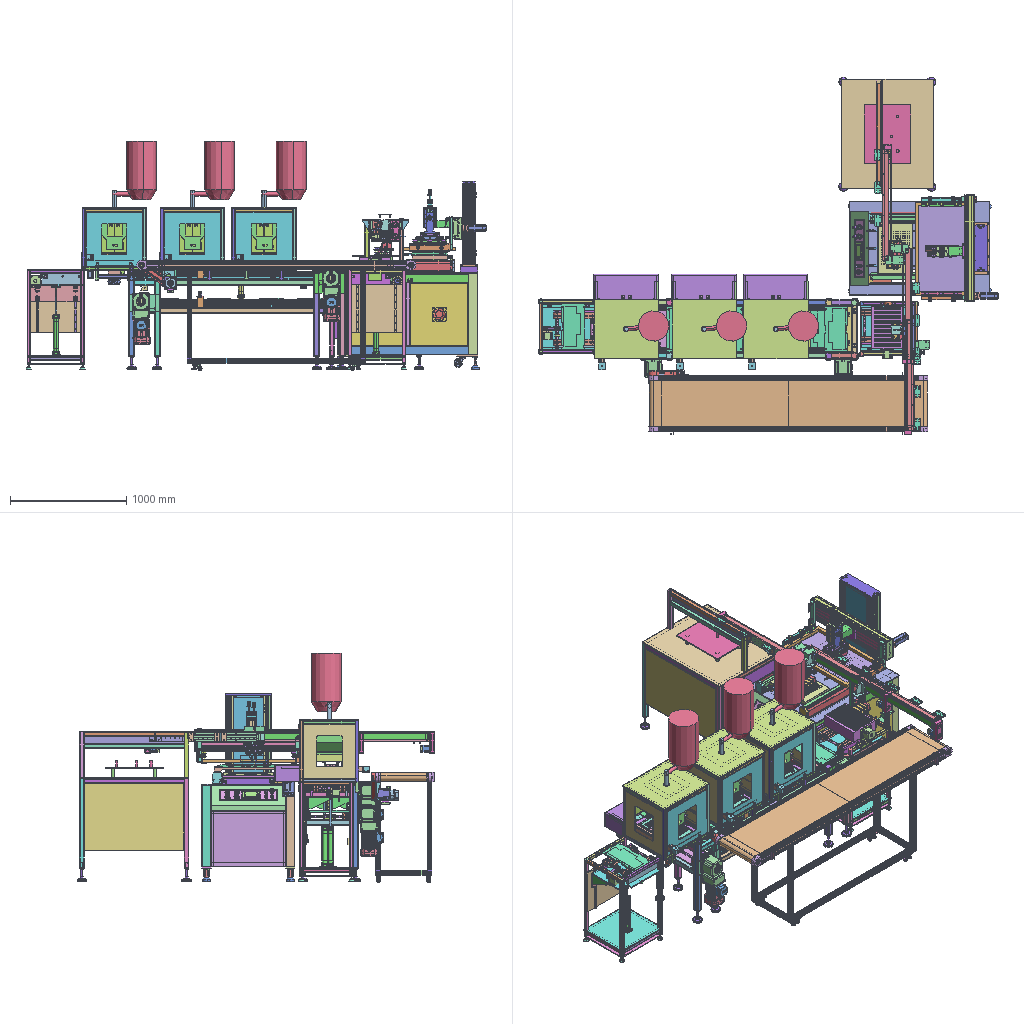Assembly | STEP file | 266 different items | 841 placed | box 3950 x 3072 x 1968 mm
Parts list (item | name | quantity | parent item | size | volume):
1 | 001. Pressure gauge (without flange) | x2 | in Circuit control assembly | 42 x 42 x 38 mm | 32331 mm3
2 | 001. Schneider red emergency stop switch XB2-BS542C | x1 | in Circuit control assembly | 40 x 40 x 49 mm | 26880 mm3
3 | 001. Schneider two-position switch XB2-BD21C | x2 | in Circuit control assembly | 28.3 x 29.2 x 44.3 mm | 13844 mm3
4 | 001. Yiweide green push-button switch EB6-BA31 | x1 | in Circuit control assembly | 28.3 x 28.3 x 27.1 mm | 9249 mm3
5 | 1.6 m_VMF01-40-4-A-001 | x27 | in 1.6米VMF01-40-2-A | 18.36 x 10.41 x 23.11 mm | 962.85 mm3
6 | 1.6 m_VMF01-40-4-A-002 | x27 | in 1.6米VMF01-40-2-A | 11.17 x 12.07 x 24.77 mm | 1310 mm3
7 | 1.6米90W | x1 | in MYT-A01-13 | 160.5 x 104 x 90 mm | 953973 mm3
8 | 1.6米B6204ZZ | x4 | in MYT-A01-13 | 14 x 47 x 47 mm | 19015 mm3
9 | 1.6米HFS8-4040-110 | x4 | in MYT-A01-13 | 40 x 40 x 800 mm | 497640 mm3
10 | 1.6米HFS8-4040-2150 | x2 | in MYT-A01-13 | 40 x 40 x 1450 mm | 901973 mm3
11 | 1.6米HFS8-4040-400 | x2 | in MYT-A01-13 | 40 x 40 x 400 mm | 248820 mm3
12 | 1.6米HFS8-4080-3000 | x2 | in MYT-A01-13 | 40 x 80 x 2230 mm | 2325189 mm3
13 | 1.6米L型片 | x4 | in MYT-A01-13 | 27 x 80 x 27 mm | 11342 mm3
14 | 1.6米VLF02-40-10-D15 | x2 | in MYT-A01-13 | 46 x 44.551 x 22 mm | 14102 mm3
15 | 1.6米托片 | x2 | in MYT-A01-13 | 49 x 32 x 36 mm | 5023 mm3
16 | 1.6米滚轮1 | x1 | in MYT-A01-13 | 70 x 486 x 70 mm | 1669260 mm3
17 | 1.6米滚轮2 | x1 | in MYT-A01-13 | 70 x 516 x 70 mm | 1674212 mm3
18 | 1.6米Belt | x1 | in MYT-A01-13 | 2391 x 398 x 76 mm | 5802047 mm3
19 | 1.6米Belt线支撑(Default) | x2 | in MYT-A01-13 | 400 x 1085 x 40 mm | 772332 mm3
20 | 1.6米Belt罩 | x1 | in MYT-A01-13 | 359.4 x 80 x 39 mm | 70115 mm3
21 | 1.6米脚轮垫块 | x4 | in MYT-A01-13 | 99 x 5 x 50 mm | 23511 mm3
22 | 1.6米轴承套 | x4 | in MYT-A01-13 | 53 x 25 x 53 mm | 15579 mm3
23 | 1.6米轴盖 | x4 | in MYT-A01-13 | 195 x 67 x 85 mm | 66626 mm3
24 | 1.6米马达罩 | x1 | in MYT-A01-13 | 145 x 105 x 42 mm | 63685 mm3
25 | 10 | x8 | in MHC-H24-2-L410 Shanglong slider, MHC-H24-2-L410 Upper隆滑块-1, MHC-H24-2-L410 Upper隆滑块-2, MHC-H24-2-L410 Upper隆滑块-3, MHC-H24-2-L410 Upper隆滑块-4, MHC-H24-2-L410 Upper隆滑块-5, MHC-H24-2-L410 Upper隆滑块-6, MHC-H24-2-L410 Upper隆滑块-7 | 32 x 18.8 x 1 mm | 485.961 mm3
26 | 11 | x8 | in MHC-H24-2-L410 Shanglong slider, MHC-H24-2-L410 Upper隆滑块-1, MHC-H24-2-L410 Upper隆滑块-2, MHC-H24-2-L410 Upper隆滑块-3, MHC-H24-2-L410 Upper隆滑块-4, MHC-H24-2-L410 Upper隆滑块-5, MHC-H24-2-L410 Upper隆滑块-6, MHC-H24-2-L410 Upper隆滑块-7 | 32 x 19.4 x 7.5 mm | 2771 mm3
27 | 12 | x8 | in MHC-H24-2-L410 Shanglong slider, MHC-H24-2-L410 Upper隆滑块-1, MHC-H24-2-L410 Upper隆滑块-2, MHC-H24-2-L410 Upper隆滑块-3, MHC-H24-2-L410 Upper隆滑块-4, MHC-H24-2-L410 Upper隆滑块-5, MHC-H24-2-L410 Upper隆滑块-6, MHC-H24-2-L410 Upper隆滑块-7 | 32 x 18.8 x 1 mm | 479.678 mm3
28 | 13 | x8 | in MHC-H24-2-L410 Shanglong slider, MHC-H24-2-L410 Upper隆滑块-1, MHC-H24-2-L410 Upper隆滑块-2, MHC-H24-2-L410 Upper隆滑块-3, MHC-H24-2-L410 Upper隆滑块-4, MHC-H24-2-L410 Upper隆滑块-5, MHC-H24-2-L410 Upper隆滑块-6, MHC-H24-2-L410 Upper隆滑块-7 | 7.302 x 8 x 6.95 mm | 149.976 mm3
29 | 200ys04 | x3 | in MYT-A01-06, MYT-A01-06-1, MYT-A01-06-2 | 199 x 143.386 x 105.972 mm | 487784 mm3
30 | 6022ZZ deep groove ball bearing MISUMI 62 | x4 | in Flat belt conveyor assembly, 平Belt输送Component-1 | 44 x 44 x 12 mm | 13685 mm3
31 | 8 | x8 | in MHC-H24-2-L410 Shanglong slider, MHC-H24-2-L410 Upper隆滑块-1, MHC-H24-2-L410 Upper隆滑块-2, MHC-H24-2-L410 Upper隆滑块-3, MHC-H24-2-L410 Upper隆滑块-4, MHC-H24-2-L410 Upper隆滑块-5, MHC-H24-2-L410 Upper隆滑块-6, MHC-H24-2-L410 Upper隆滑块-7 | 34 x 19.5 x 39.8 mm | 15652 mm3
32 | 866-BDO024-91-11A_default_machined_ | x9 | in 866-BDO024-95-00A_material release position, 866-BDO024-95-00A_放料位-1, 866-BDO024-95-00A_放料位-2 | 90 x 65 x 100 mm | 167392 mm3
33 | 866-BDO024-93-03A | x3 | in 866-BDO024-95-00A_material release position, 866-BDO024-95-00A_放料位-1, 866-BDO024-95-00A_放料位-2 | 80 x 61.5 x 14 mm | 48551 mm3
34 | 866-BDO024-93-04A | x3 | in 866-BDO024-95-00A_material release position, 866-BDO024-95-00A_放料位-1, 866-BDO024-95-00A_放料位-2 | 80 x 57 x 75 mm | 148857 mm3
35 | 866-BDO024-93-10A | x3 | in 866-BDO024-95-00A_material release position, 866-BDO024-95-00A_放料位-1, 866-BDO024-95-00A_放料位-2 | 16 x 35 x 9 mm | 897.701 mm3
36 | 866-BDO024-93-11A | x9 | in 866-BDO024-95-00A_material release position, 866-BDO024-95-00A_放料位-1, 866-BDO024-95-00A_放料位-2 | 25 x 6 x 3 mm | 420.548 mm3
37 | 866-BDO024-93-12A | x6 | in 866-BDO024-95-00A_material release position, 866-BDO024-95-00A_放料位-1, 866-BDO024-95-00A_放料位-2 | 80 x 61.5 x 20 mm | 50514 mm3
38 | 866-BDO024-95-01A_default | x3 | in 866-BDO024-95-00A_material release position, 866-BDO024-95-00A_放料位-1, 866-BDO024-95-00A_放料位-2 | 954 x 15 x 80 mm | 1055067 mm3
39 | 866-BDO024-95-03A | x3 | in 866-BDO024-95-00A_material release position, 866-BDO024-95-00A_放料位-1, 866-BDO024-95-00A_放料位-2 | 954 x 8 x 56 mm | 95867 mm3
40 | 866-BDO024-95-04A | x3 | in 866-BDO024-95-00A_material release position, 866-BDO024-95-00A_放料位-1, 866-BDO024-95-00A_放料位-2 | 942 x 56.5 x 13.5 mm | 95046 mm3
41 | 866-BDO024-95-05A | x3 | in 866-BDO024-95-00A_material release position, 866-BDO024-95-00A_放料位-1, 866-BDO024-95-00A_放料位-2 | 180 x 63 x 20 mm | 101274 mm3
42 | 866-BDO024-95-06A | x3 | in 866-BDO024-95-00A_material release position, 866-BDO024-95-00A_放料位-1, 866-BDO024-95-00A_放料位-2 | 66 x 46.5 x 183 mm | 47761 mm3
43 | 866-BDO024-95-07A_default | x3 | in 866-BDO024-95-00A_material release position, 866-BDO024-95-00A_放料位-1, 866-BDO024-95-00A_放料位-2 | 13.5 x 56.5 x 954 mm | 96451 mm3
44 | 866-BDO024-96-03A_default | x3 | in 866-BDO024-96-00A_material release position, 866-BDO024-96-00A_放料位-1, 866-BDO024-96-00A_放料位-2 | 148.5 x 75 x 45.5 mm | 21210 mm3
45 | 9 | x8 | in MHC-H24-2-L410 Shanglong slider, MHC-H24-2-L410 Upper隆滑块-1, MHC-H24-2-L410 Upper隆滑块-2, MHC-H24-2-L410 Upper隆滑块-3, MHC-H24-2-L410 Upper隆滑块-4, MHC-H24-2-L410 Upper隆滑块-5, MHC-H24-2-L410 Upper隆滑块-6, MHC-H24-2-L410 Upper隆滑块-7 | 32 x 19.4 x 7.5 mm | 2771 mm3
46 | 90yt01-18 | x1 | in Speed control motor assembly | - | -
47 | AC motor fixing | x1 | in Speed control motor assembly | 100 x 250 x 8 mm | 168414 mm3
48 | AJC-D48-M10-L80 | x8 | in AJC-D48-M10-L80 leveling foot cup Shanglong 17.2, AJC-D48-M10-L80 leveling foot cup Shanglong 17.2-1, AJC-D48-M10-L80 leveling foot cup Shanglong 17.2-2, AJC-D48-M10-L80 leveling foot cup Shanglong 17.2-3, AJC-D48-M10-L80 leveling foot cup Shanglong 17.2-4, AJC-D48-M10-L80 leveling foot cup Shanglong 17.2-5, AJC-D48-M10-L80 leveling foot cup Shanglong 17.2-6, AJC-D48-M10-L80 leveling foot cup Shanglong 17.2-7 | 48 x 102 x 48 mm | 30151 mm3
49 | AKQ41-G-Z-6065 | x12 | in MYT-A01-06, MYT-A01-06-1, MYT-A01-06-2 | 60 x 13.5 x 65 mm | 16186 mm3
50 | Air cylinder ACQJ-25X35-20_4_1-5 | x2 | in New head | 40 x 151.001 x 42 mm | 88087 mm3
51 | BAF629ZZ-E | x6 | in MYT-A01-06, MYT-A01-06-1, MYT-A01-06-2 | 8 x 26 x 26 mm | 3194 mm3
52 | BRTA-20 pillow block bearing Shanglong | x6 | in MYT-A01-00, MYT-A01-03, MYT-A01-03-1 | 37 x 73.015 x 127 mm | 112012 mm3
53 | BTL-01-32-0 | x4 | in MYT-A01-01, MYT-A01-01-1, MYT-A01-01-2, MYT-A01-01-3 | 40 x 32 x 32 mm | 13951 mm3
54 | Ball screw 4R16-16S2-DFSH-920-982-0.05(R)_HIWIN | x3 | in 866-BDO024-95-00A_material release position, 866-BDO024-95-00A_放料位-1, 866-BDO024-95-00A_放料位-2 | 982 x 16 x 16 mm | 189994 mm3
55 | Ball screw 4R16-16S2-DFSH-920-982-0.05(S)_HIWEI_default | x3 | in 866-BDO024-95-00A_material release position, 866-BDO024-95-00A_放料位-1, 866-BDO024-95-00A_放料位-2 | 38 x 53 x 48 mm | 38522 mm3
56 | Bearing B6000ZZ_MISUMI | x3 | in 866-BDO024-95-00A_material release position, 866-BDO024-95-00A_放料位-1, 866-BDO024-95-00A_放料位-2 | 8 x 26 x 26 mm | 2470 mm3
57 | Bearing B6201ZZNR_MISUMI | x6 | in 866-BDO024-95-00A_material release position, 866-BDO024-95-00A_放料位-1, 866-BDO024-95-00A_放料位-2 | 10 x 36.7 x 36.7 mm | 5407 mm3
58 | Blade clamp | x1 | in Blade-modified | 250 x 36 x 53 mm | 139062 mm3
59 | Blade fixing rod | x2 | in Blade-modified, 回墨刀-350 | 230 x 30 x 30 mm | 83181 mm3
60 | Blade holder 1 | x4 | in New head | 45 x 20 x 75 mm | 28350 mm3
61 | C-type retaining ring STWS10_MISUMI_default | x3 | in 866-BDO024-95-00A_material release position, 866-BDO024-95-00A_放料位-1, 866-BDO024-95-00A_放料位-2 | 12 x 1 x 14.09 mm | 51.059 mm3
62 | CA2F40-50Z_0_0_0_ | x1 | in MYT-A01-07 | 196 x 71 x 100 mm | 325906 mm3
63 | CA2G40-250Z_0_0_0_ | x2 | in MYT-A01-05, MYT-A01-05-1 | 624.042 x 71 x 100 mm | 473090 mm3
64 | CJ2KD16-45S_0_0_0_ | x3 | in MYT-A01-06, MYT-A01-06-1, MYT-A01-06-2 | 149 x 18.3 x 22.7 mm | 23348 mm3
65 | CQ2F16-20D_0_0_0_ | x6 | in MYT-A01-08, MYT-A01-08-1, MYT-A01-08-2, MYT-A01-08-3, MYT-A01-08-4 | 52 x 30 x 55 mm | 31057 mm3
66 | CQ2G32-50DZ_0_0_0_ | x3 | in MYT-A01-11, MYT-A01-11-1 | 88 x 51 x 65 mm | 108830 mm3
67 | Caster plate | x4 | in CMAZ40-N ultra-light caster, CMAZ40-N脚轮超轻载-1, CMAZ40-N脚轮超轻载-2, CMAZ40-N脚轮超轻载-3 | 50 x 6.8 x 69 mm | 8896 mm3
68 | Column | x2 | in Vertical arm unit | 107.4 x 51 x 700 mm | 1396461 mm3
69 | Column base plate | x1 | in Vertical arm unit | 450 x 150 x 15 mm | 884150 mm3
70 | Column cover plate | x1 | in Vertical arm unit | 400 x 107.5 x 15 mm | 621699 mm3
71 | Connecting bolt | x2 | in New head | 14 x 16.166 x 28 mm | 2024 mm3
72 | profile cover | x2 | in Blade-modified | 8 x 30 x 30 mm | 5851 mm3
73 | rotating shaft | x2 | in Blade clamp assembly, 刮刀夹组合-1 | 20 x 20 x 114 mm | 37100 mm3
74 | Crossbeam front guard plate | x1 | in Printing crossbeam unit | 98 x 8 x 898 mm | 149433 mm3
75 | Crossbeam slider connecting plate | x1 | in Printing crossbeam unit | 130 x 125 x 21 mm | 162372 mm3
76 | Double-speed chain return rail VMH01-BS25-C206B Yihda 124-0 | x6 | in MYT-A01-00, MYT-A01-03, MYT-A01-03-1 | 34 x 56.925 x 56.925 mm | 78739 mm3
77 | Driven wheel | x1 | in Driven wheel assembly | 42.62 x 42.62 x 24.392 mm | 14671 mm3
78 | Driven wheel shaft^Driven wheel assembly | x1 | in Driven wheel assembly | 16 x 16 x 66 mm | 7306 mm3
79 | Driving wheel | x1 | in Printing motor assembly | 42.62 x 42.62 x 24.392 mm | 18419 mm3
80 | E-LME12-d10 | x4 | in MYT-A01-07 | 29 x 40 x 40 mm | 8759 mm3
81 | E-WAC53-D80-M16-L125 | x12 | in MYT-A01-00, MYT-A01-09 | 80 x 165 x 80 mm | 107171 mm3
82 | EME01-W50-L0.793 flat belt Yihda 113 | x4 | in Flat belt conveyor assembly, 平Belt输送Component-1 | 362.8 x 62.8 x 50 mm | 76314 mm3
83 | ENE11-D60-N20-L50-X14-Y12-Z5 flat belt pulley Yihda 171 | x4 | in Flat belt conveyor assembly, 平Belt输送Component-1 | 60 x 60 x 50 mm | 110095 mm3
84 | ENJ11-D60-d20-L50-X14-Y12-Z5 flat belt idler Yihda 271 | x8 | in Flat belt idler assembly, 平带惰轮Component-1, 平带惰轮Component-2, 平带惰轮Component-3, 平带惰轮Component-4, 平带惰轮Component-5, 平带惰轮Component-6, 平带惰轮Component-7 | 60 x 60 x 50 mm | 111446 mm3
85 | Electromagnet | x2 | in Dual platform unit | 25 x 25 x 15 mm | 6939 mm3
86 | Five-star handle (with gland) (M10_40_40) | x3 | in Right screen clamp assembly^Screen assembly_PS-3045E-LDJ | 38.486 x 37.046 x 70.083 mm | 22563 mm3
87 | Five-star handle (with gland) 2 (M10_40_40) | x3 | in Right screen clamp assembly^Screen assembly_PS-3045E-LDJ2 | 38.486 x 37.046 x 70.083 mm | 22563 mm3
88 | Fixed seat | x1 | in New head | 105 x 75 x 160 mm | 453829 mm3
89 | Flat belt conveyor base plate | x2 | in Flat belt conveyor assembly, 平Belt输送Component-1 | 463 x 393.9 x 10 mm | 1773598 mm3
90 | Flat belt drive shaft | x6 | in Flat belt conveyor assembly, 平Belt输送Component-1 | 283.4 x 22 x 22 mm | 95567 mm3
91 | Flat belt motor mounting plate | x2 | in Flat belt conveyor assembly, 平Belt输送Component-1 | 86 x 101 x 12 mm | 83890 mm3
92 | Flat belt mounting plate | x2 | in Flat belt conveyor assembly, 平Belt输送Component-1 | 355 x 95 x 16 mm | 507779 mm3
93 | Floating joint | x4 | in Flat belt conveyor assembly, New head, 平Belt输送Component-1 | 20 x 38 x 33 mm | 13622 mm3
94 | Floating joint mounting plate | x2 | in Flat belt conveyor assembly, 平Belt输送Component-1 | 38 x 75 x 18 mm | 24096 mm3
95 | Flow limiter AS2201F-01-06_SMC_22-01-06 | x6 | in 866-BDO024-96-00A_material release position, 866-BDO024-96-00A_放料位-1, 866-BDO024-96-00A_放料位-2 | 27.5 x 36.1 x 14.2 mm | 4282 mm3
96 | Foot caster | x4 | in Frame unit | 60 x 96 x 114 mm | 163326 mm3
97 | Foot pad shim | x4 | in Foot cup, 地脚杯-1, 地脚杯-2, 地脚杯-3 | 65 x 65 x 35 mm | 88423 mm3
98 | Foot screw | x4 | in Foot cup, 地脚杯-1, 地脚杯-2, 地脚杯-3 | 20 x 118 x 20 mm | 31335 mm3
99 | Frame | x1 | in Frame unit | 800 x 785 x 1200 mm | 26873154 mm3
100 | Gland cover^Driven wheel assembly | x1 | in Driven wheel assembly | 16 x 16 x 2 mm | 364.163 mm3
101 | Guide rail HGH15 (HGH15 rail) | x4 | in Platform guide assembly, Flat导向Component-1 | 15 x 15 x 760 mm | 145713 mm3
102 | Guide rail mounting plate | x2 | in MYT-A01-05, MYT-A01-05-1 | 493 x 410 x 12 mm | 2425560 mm3
103 | Guide rail stopper | x1 | in Dual platform unit | 85 x 90 x 35 mm | 250787 mm3
104 | Guide rail stopper 111 | x1 | in Dual platform unit | 85 x 90 x 35 mm | 251654 mm3
105 | Guide rail stopper 2 | x1 | in Dual platform unit | 85 x 90 x 35 mm | 251196 mm3
106 | Guide rail stopper 22 | x1 | in Dual platform unit | 85 x 90 x 35 mm | 251196 mm3
107 | HGH15 guide rail 2 (HGH15 rail) | x2 | in Vertical arm unit | 15 x 15 x 668 mm | 127557 mm3
108 | HGH15 guide rail 3 (HGH15 rail) | x2 | in Printing crossbeam unit | 15 x 15 x 800 mm | 153607 mm3
109 | HGH15CA slider ( HGH15CA) | x3 | in Printing crossbeam unit | 34 x 23.7 x 61.4 mm | 37112 mm3
110 | HGH25 rail | x6 | in MYT-A01-06, MYT-A01-06-1, MYT-A01-06-2 | 23 x 22 x 506 mm | 212116 mm3
111 | HGH25 slider | x12 | in MYT-A01-06, MYT-A01-06-1, MYT-A01-06-2 | 48 x 34.5 x 82 mm | 100220 mm3
112 | HTBNV355-S5M-250 high-torque timing belt S5M MISUMI 24 | x2 | in Flat belt conveyor assembly, 平Belt输送Component-1 | 150.61 x 58.11 x 25 mm | 18064 mm3
113 | HTPA20S5M150-A-N15 | x2 | in MYT-A01-13, Speed control motor assembly | - | -
114 | HTPA34S5M250-A-N12 high-torque timing pulley MISUMI 110 | x2 | in Flat belt conveyor assembly, 平Belt输送Component-1 | 32.194 x 61 x 61 mm | 63360 mm3
115 | HTPA34S5M250-A-N22 high-torque timing pulley MISUMI 110 | x2 | in Flat belt conveyor assembly, 平Belt输送Component-1 | 32.194 x 61 x 61 mm | 54521 mm3
116 | Head fixing plate | x1 | in New head | 130 x 130 x 20 mm | 311924 mm3
117 | Head front cover plate | x1 | in New head | 84 x 175 x 10 mm | 137909 mm3
118 | Hinge bracket 40-40 | x2 | in Vertical arm unit | 40 x 40 x 10 mm | 8942 mm3
119 | In/out guide rail cover plate 1 | x2 | in Dual platform unit | 57 x 52 x 800 mm | 124915 mm3
120 | In/out guide rail cover plate 2 | x2 | in Dual platform unit | 20 x 90 x 800 mm | 180213 mm3
121 | Insert strip | x2 | in Vertical arm unit | 250 x 10 x 20 mm | 48396 mm3
122 | JHSTM86-1.8-S-65-3 stepper motor MISUMI 657 | x3 | in Flat belt conveyor assembly, 平Belt输送Component-1 | 86 x 116 x 96.85 mm | 438131 mm3
123 | Label: fan 105×105 | x4 | in Frame unit | 120 x 120 x 39 mm | 155922 mm3
124 | Label: micrometer range 25mm diameter 12 new | x6 | in Micrometer fine-adjustment assembly new, 千分尺微调Component新-1, 千分尺微调Component新-2, 千分尺微调Component新-3, 千分尺微调Component新-4, 千分尺微调Component新-5 | 113 x 18 x 18 mm | 13941 mm3
125 | Lift frame (default_machined_) | x2 | in MYT-A01-05, MYT-A01-05-1 | 460 x 814 x 493 mm | 5738734 mm3
126 | Linear rail MR15WLSS1V1H-880L-20-20-I(R)_CPC_default | x3 | in 866-BDO024-95-00A_material release position, 866-BDO024-95-00A_放料位-1, 866-BDO024-95-00A_放料位-2 | 880 x 9.5 x 42 mm | 319876 mm3
127 | Linear rail MR15WLSS1V1H-880L-20-20-I(S)_CPC_default | x3 | in 866-BDO024-95-00A_material release position, 866-BDO024-95-00A_放料位-1, 866-BDO024-95-00A_放料位-2 | 74.5 x 12 x 60 mm | 35281 mm3
128 | Lock block wdl | x4 | in Blade clamp assembly, 刮刀夹组合-1 | 18 x 35 x 12 mm | 5552 mm3
129 | Lock nut FUNT12_MISUMI | x3 | in 866-BDO024-95-00A_material release position, 866-BDO024-95-00A_放料位-1, 866-BDO024-95-00A_放料位-2 | 5.4 x 22 x 22 mm | 932.86 mm3
130 | M12 | x8 | in Flat belt idler assembly, 平带惰轮Component-1, 平带惰轮Component-2, 平带惰轮Component-3, 平带惰轮Component-4, 平带惰轮Component-5, 平带惰轮Component-6, 平带惰轮Component-7 | 19 x 21.939 x 10 mm | 2601 mm3
131 | M12-L85-0 | x2 | in MYT-A01-02, MYT-A01-02-1 | 19 x 21.939 x 92.5 mm | 11946 mm3
132 | M8 M6 M10(M6_45_40) | x2 | in Right screen clamp assembly^Screen assembly_PS-3045E-LDJ | 77.136 x 22 x 82.928 mm | 11260 mm3
133 | M8 M6 M102(M6_45_40) | x2 | in Right screen clamp assembly^Screen assembly_PS-3045E-LDJ2 | 77.136 x 22 x 82.928 mm | 11260 mm3
134 | MHC-H24-2-L410 Shanglong guide rail | x4 | in MYT-A01-05, MYT-A01-05-1 | 15 x 12.5 x 410 mm | 68741 mm3
135 | MJ45 HS120 Y-axis motor | x3 | in MJ45 module, MJ45模组-1, MJ45模组-2 | 51.6 x 60.6 x 90 mm | 170208 mm3
136 | MJ45 coupling | x3 | in MJ45 module, MJ45模组-1, MJ45模组-2 | 35 x 50 x 35 mm | 41891 mm3
137 | MJ45 motor base fixing | x3 | in MJ45 module, MJ45模组-1, MJ45模组-2 | 70.4 x 54.4 x 90.4 mm | 105657 mm3
138 | MJ45 motor support seat | x3 | in MJ45 module, MJ45模组-1, MJ45模组-2 | 89 x 58 x 62.5 mm | 152707 mm3
139 | MJ45 slide rail | x3 | in MJ45 module, MJ45模组-1, MJ45模组-2 | 45 x 49 x 620 mm | 255112 mm3
140 | MJ45 slider | x3 | in MJ45 module, MJ45模组-1, MJ45模组-2 | 104 x 90 x 20 mm | 164549 mm3
141 | MJ45 standard foot | x6 | in MJ45 module, MJ45模组-1, MJ45模组-2 | 64 x 68 x 10 mm | 31336 mm3
142 | MYT-A01-P01(default_machined_) | x1 | in MYT-A01-00 | 1860 x 514 x 715 mm | 13979355 mm3
143 | MYT-A01-P02 | x4 | in MYT-A01-03, MYT-A01-03-1 | 43 x 72 x 1840 mm | 1165090 mm3
144 | MYT-A01-P03 | x4 | in MYT-A01-03, MYT-A01-03-1 | - | 527480 mm3
145 | MYT-A01-P07 | x9 | in MYT-A01-00 | 390 x 200 x 15 mm | 1098768 mm3
146 | MYT-A01-P10 | x2 | in MYT-A01-03, MYT-A01-03-1 | 20 x 20 x 366.3 mm | 97502 mm3
147 | MYT-A01-P11 | x4 | in MYT-A01-02, MYT-A01-02-1 | 40 x 45 x 10 mm | 12427 mm3
148 | MYT-A01-P12 | x2 | in MYT-A01-02, MYT-A01-02-1 | 100 x 40 x 10 mm | 37260 mm3
149 | MYT-A01-P13 | x1 | in MYT-A01-00 | 100 x 70 x 10 mm | 43994 mm3
150 | MYT-A01-P14(Default_machined_) | x3 | in MYT-A01-06, MYT-A01-06-1, MYT-A01-06-2 | 550 x 666 x 625 mm | 6400187 mm3
151 | MYT-A01-P15 | x3 | in MYT-A01-06, MYT-A01-06-1, MYT-A01-06-2 | 506 x 330 x 15 mm | 328468 mm3
152 | MYT-A01-P16 | x3 | in MYT-A01-06, MYT-A01-06-1, MYT-A01-06-2 | 150 x 50 x 10 mm | 59016 mm3
153 | MYT-A01-P17 | x3 | in MYT-A01-06, MYT-A01-06-1, MYT-A01-06-2 | 50 x 50 x 40 mm | 38280 mm3
154 | MYT-A01-P18 | x3 | in MYT-A01-06, MYT-A01-06-1, MYT-A01-06-2 | 150 x 110 x 10 mm | 165000 mm3
155 | MYT-A01-P19 | x3 | in MYT-A01-06, MYT-A01-06-1, MYT-A01-06-2 | 300 x 352 x 300 mm | 782143 mm3
156 | MYT-A01-P21 | x6 | in MYT-A01-06, MYT-A01-06-1, MYT-A01-06-2 | 300 x 65 x 82 mm | 87000 mm3
157 | MYT-A01-P22 | x3 | in MYT-A01-06, MYT-A01-06-1, MYT-A01-06-2 | 80 x 2 x 30 mm | 4800 mm3
158 | MYT-A01-P23 | x3 | in MYT-A01-06, MYT-A01-06-1, MYT-A01-06-2 | 489 x 469 x 18 mm | 480238 mm3
159 | MYT-A01-P24 | x6 | in MYT-A01-06, MYT-A01-06-1, MYT-A01-06-2 | 448 x 469 x 18 mm | 435629 mm3
160 | MYT-A01-P25 | x3 | in MYT-A01-06, MYT-A01-06-1, MYT-A01-06-2 | 550 x 220 x 150 mm | 518815 mm3
161 | MYT-A01-P26 | x6 | in MYT-A01-06, MYT-A01-06-1, MYT-A01-06-2 | 242 x 348 x 5 mm | 421080 mm3
162 | MYT-A01-P27 | x3 | in MYT-A01-06, MYT-A01-06-1, MYT-A01-06-2 | 260 x 410 x 5 mm | 444533 mm3
163 | MYT-A01-P28 | x1 | in MYT-A01-07 | 130 x 500 x 10 mm | 619024 mm3
164 | MYT-A01-P29 | x1 | in MYT-A01-07 | 200 x 100 x 10 mm | 196251 mm3
165 | MYT-A01-P30 | x5 | in MYT-A01-08, MYT-A01-08-1, MYT-A01-08-2, MYT-A01-08-3, MYT-A01-08-4 | 63 x 103 x 50 mm | 24306 mm3
166 | MYT-A01-P31 | x5 | in MYT-A01-08, MYT-A01-08-1, MYT-A01-08-2, MYT-A01-08-3, MYT-A01-08-4 | 12 x 12 x 30 mm | 3393 mm3
167 | MYT-A01-P32(Default_machined_) | x1 | in MYT-A01-09 | 940 x 790 x 1170 mm | 12412396 mm3
168 | MYT-A01-P33 | x4 | in MYT-A01-09 | 30 x 30 x 260 mm | 183783 mm3
169 | MYT-A01-P34 | x1 | in MYT-A01-09 | 500 x 400 x 70 mm | 2065250 mm3
170 | MYT-A01-P35 | x1 | in MYT-A01-09 | 420 x 300 x 10 mm | 1260000 mm3
171 | MYT-A01-P36 | x2 | in MYT-A01-09 | 860 x 580 x 15 mm | 1590637 mm3
172 | MYT-A01-P37 | x2 | in MYT-A01-09 | 710 x 580 x 15 mm | 1319701 mm3
173 | MYT-A01-P39 | x3 | in MYT-A01-11, MYT-A01-11-1 | 75 x 100 x 90 mm | 190302 mm3
174 | MYT-A01-P40(Default_machined_) | x1 | - | 460 x 443 x 30 mm | 846858 mm3
175 | MYT-A01-P41 | x1 | - | 80 x 100 x 5 mm | 40000 mm3
176 | MYT-A01-P42 | x1 | - | 120 x 190 x 10 mm | 228000 mm3
177 | Magnet block | x2 | in Dual platform unit | 25 x 25 x 20 mm | 10144 mm3
178 | Main beam | x1 | in Printing crossbeam unit | 80 x 900 x 190 mm | 4670487 mm3
179 | Main beam baffle 1 | x1 | in Printing crossbeam unit | 80 x 190 x 10 mm | 151750 mm3
180 | Main beam baffle 2 | x1 | in Printing crossbeam unit | 80 x 190 x 10 mm | 151750 mm3
181 | Micrometer head fixing seat new | x6 | in Micrometer fine-adjustment assembly new, 千分尺微调Component新-1, 千分尺微调Component新-2, 千分尺微调Component新-3, 千分尺微调Component新-4, 千分尺微调Component新-5 | 40 x 18 x 17 mm | 4623 mm3
182 | Mirrored MJ45 motor support seat | x3 | in MJ45 module, MJ45模组-1, MJ45模组-2 | 45 x 58 x 62.5 mm | 148250 mm3
183 | Mobile suction-cup manipulator | x4 | - | 120 x 117.5 x 141 mm | 84416 mm3
184 | Panasonic A4 servo motor (400W220V) | x1 | in Printing motor assembly | 184.5 x 60 x 60 mm | 493168 mm3
185 | Panel | x1 | in Circuit control assembly | 500 x 125 x 1.5 mm | 67047 mm3
186 | Part 10 | x3 | in MYT-A01-06, MYT-A01-06-1, MYT-A01-06-2 | 100 x 60 x 360 mm | 410000 mm3
187 | Part 1^Dual platform unit | x2 | in Dual platform unit | 35 x 35 x 40 mm | 24064 mm3
188 | Part 1^New head | x1 | in New head | 60 x 75 x 117 mm | 523169 mm3
189 | Part 2^Frame unit | x4 | in Frame unit | 498 x 538 x 13.5 mm | 425403 mm3
190 | Part 3^Frame unit | x2 | in Frame unit | 638 x 538 x 13.5 mm | 554979 mm3
191 | Part 60 | x1 | - | 260 x 100 x 360 mm | 9327526 mm3
192 | Part 9 | x3 | in MYT-A01-06, MYT-A01-06-1, MYT-A01-06-2 | 32 x 20 x 300 mm | 179124 mm3
193 | Platform 1 (default) | x1 | in Platform assembly 1 | 435 x 300 x 30 mm | 1924051 mm3
194 | Platform 1 base plate | x1 | in Platform 1 unit | 448 x 300 x 15 mm | 2016000 mm3
195 | Platform 1 slider plate 1 | x1 | in Slider assembly 1 | 34 x 300 x 50 mm | 195000 mm3
196 | Platform 1 slider plate 2 | x1 | in Slider assembly 2 | 71.5 x 300 x 34 mm | 220800 mm3
197 | Platform 2 | x1 | in Platform assembly 2 | 585 x 300 x 30 mm | 2256819 mm3
198 | Platform 2 base plate | x1 | in Platform 2 unit | 585 x 300 x 30 mm | 2764800 mm3
199 | Platform 2 slider plate 1 | x1 | in Platform 2 unit | 35 x 33 x 300 mm | 183000 mm3
200 | Platform 2 slider plate 2 | x1 | in Platform 2 unit | 35 x 124 x 300 mm | 337200 mm3
201 | Platform guide seat (default) | x2 | in Platform guide assembly, Flat导向Component-1 | 45 x 47 x 770 mm | 1483790 mm3
202 | Pressure regulating valve AR2000 | x2 | in Circuit control assembly | 57 x 39.5 x 96 mm | 107387 mm3
203 | Printing cylinder fixing plate | x1 | in New head | 84 x 105 x 15 mm | 114533 mm3
204 | Printing fixing plate | x2 | in New head | 88 x 206 x 22 mm | 274808 mm3
205 | Reinforcing rib | x6 | in Flat belt conveyor assembly, 平Belt输送Component-1 | 181.9 x 96 x 10 mm | 113102 mm3
206 | Return squeegee | x1 | in 回墨刀-350 | 49.219 x 85.9 x 280 mm | 99161 mm3
207 | Right flat belt mounting plate | x2 | in Flat belt conveyor assembly, 平Belt输送Component-1 | 355 x 95 x 16 mm | 507779 mm3
208 | SCD11-D10-L80-M6 | x4 | in MYT-A01-07 | 80 x 10 x 10 mm | 6034 mm3
209 | SLMNA10 | x8 | in AJC-D48-M10-L80 leveling foot cup Shanglong 17.2, AJC-D48-M10-L80 leveling foot cup Shanglong 17.2-1, AJC-D48-M10-L80 leveling foot cup Shanglong 17.2-2, AJC-D48-M10-L80 leveling foot cup Shanglong 17.2-3, AJC-D48-M10-L80 leveling foot cup Shanglong 17.2-4, AJC-D48-M10-L80 leveling foot cup Shanglong 17.2-5, AJC-D48-M10-L80 leveling foot cup Shanglong 17.2-6, AJC-D48-M10-L80 leveling foot cup Shanglong 17.2-7 | - | -
210 | SLMNA12-0 | x4 | in MYT-A01-01, MYT-A01-01-1, MYT-A01-01-2, MYT-A01-01-3 | - | -
211 | Screen clamp | x1 | in Right screen clamp assembly^Screen assembly_PS-3045E-LDJ | 345 x 65 x 40 mm | 196764 mm3
212 | Screen clamp 2 | x1 | in Right screen clamp assembly^Screen assembly_PS-3045E-LDJ2 | 345 x 65 x 40 mm | 196764 mm3
213 | Screen clamp adjusting cap | x2 | in Screen clamp adjusting body, 网夹调节体-1 | 16 x 16 x 4 mm | 701.903 mm3
214 | Screen clamp adjusting cap 2 | x2 | in Screen clamp adjusting body 2, Screen clamp adjusting body 2-1 | 16 x 16 x 4 mm | 701.903 mm3
215 | Screen clamp adjusting handle | x2 | in Screen clamp adjusting body, 网夹调节体-1 | 28 x 28 x 57 mm | 11437 mm3
216 | Screen clamp adjusting handle 2 | x2 | in Screen clamp adjusting body 2, Screen clamp adjusting body 2-1 | 28 x 28 x 57 mm | 11437 mm3
217 | Screen clamp adjusting plate^Right screen clamp assembly_Screen assembly_PS-3045E-LDJ2 | x2 | in Right screen clamp assembly^Screen assembly_PS-3045E-LDJ, Right screen clamp assembly^Screen assembly_PS-3045E-LDJ2 | 40 x 285.5 x 31 mm | 297627 mm3
218 | Screen clamp adjusting rod | x2 | in Screen clamp adjusting body, 网夹调节体-1 | 22 x 22 x 52.5 mm | 8516 mm3
219 | Screen clamp adjusting rod 2 | x2 | in Screen clamp adjusting body 2, Screen clamp adjusting body 2-1 | 22 x 22 x 52.5 mm | 8516 mm3
220 | Screen clamp fixing plate^Right screen clamp assembly_Screen assembly_PS-3045E-LDJ | x1 | in Right screen clamp assembly^Screen assembly_PS-3045E-LDJ | 30 x 64.5 x 350 mm | 453768 mm3
221 | Screen clamp fixing plate^Right screen clamp assembly_Screen assembly_PS-3045E-LDJ2 | x1 | in Right screen clamp assembly^Screen assembly_PS-3045E-LDJ2 | 30 x 64.5 x 350 mm | 452377 mm3
222 | Screen clamp lock bolt | x3 | in Right screen clamp assembly^Screen assembly_PS-3045E-LDJ | 24 x 14 x 27.713 mm | 4195 mm3
223 | Screen clamp lock bolt 2 | x3 | in Right screen clamp assembly^Screen assembly_PS-3045E-LDJ2 | 24 x 14 x 27.713 mm | 4195 mm3
224 | Screen clamp lock nut | x2 | in Screen clamp adjusting body, 网夹调节体-1 | 28 x 28 x 16 mm | 7694 mm3
225 | Screen clamp lock nut 00 | x3 | in Right screen clamp assembly^Screen assembly_PS-3045E-LDJ | 27.713 x 4.5 x 24 mm | 1162 mm3
226 | Screen clamp lock nut 002 | x3 | in Right screen clamp assembly^Screen assembly_PS-3045E-LDJ2 | 27.713 x 4.5 x 24 mm | 1162 mm3
227 | Screen clamp lock nut 2 | x2 | in Screen clamp adjusting body 2, Screen clamp adjusting body 2-1 | 28 x 28 x 16 mm | 7694 mm3
228 | Screen plate | x1 | in Screen assembly^PS-3045E-LDJ | - | -
229 | Sensor EE-SX672_OMRON_default | x9 | in 866-BDO024-95-00A_material release position, 866-BDO024-95-00A_放料位-1, 866-BDO024-95-00A_放料位-2 | 13.7 x 38.4 x 26 mm | 2958 mm3
230 | Servo motor MSMD022P1U_Panasonic_default | x3 | in 866-BDO024-95-00A_material release position, 866-BDO024-95-00A_放料位-1, 866-BDO024-95-00A_放料位-2 | 60 x 110 x 109 mm | 279096 mm3
231 | Servo motor gearbox (PL60-8) | x1 | in Printing motor assembly | 60 x 60 x 115 mm | 234745 mm3
232 | Slider HGH15CA ( HGH15CA) | x8 | in Platform 2 unit, Slider assembly 1, Slider assembly 2 | 34 x 23.7 x 61.4 mm | 37112 mm3
233 | Slider connecting plate | x2 | in Platform 2 unit | 300 x 12 x 45 mm | 136500 mm3
234 | Squeegee pressure rubber pad | x2 | in Printing adjusting handle, 印刷调节手柄-1 | 23 x 23 x 7.5 mm | 1962 mm3
235 | Squeegee rubber | x1 | in Blade-modified | 47 x 9 x 250 mm | 105750 mm3
236 | TWH-S-32x20-K F-1-G _-0 | x1 | in MYT-A01-04 | 67 x 114 x 67 mm | 155824 mm3
237 | TWH-S-32x20-K F-1-P_r-0 | x1 | in MYT-A01-04 | 55.5 x 118.212 x 35.25 mm | 58863 mm3
238 | Timing belt TTBU325T5-150_MISUMI | x3 | in 866-BDO024-95-00A_material release position, 866-BDO024-95-00A_放料位-1, 866-BDO024-95-00A_放料位-2 | 145.88 x 43.38 x 15 mm | 5072 mm3
239 | Timing belt tensioner block^X moving platform_PS-3045E-LDJ | x1 | in Driven wheel assembly | 50 x 40 x 16 mm | 21271 mm3
240 | Timing pulley TTPA26T5150-A-N10_MISUMI_default | x3 | in 866-BDO024-95-00A_material release position, 866-BDO024-95-00A_放料位-1, 866-BDO024-95-00A_放料位-2 | 22.642 x 48 x 48 mm | 27102 mm3
241 | Timing pulley TTPA26T5150-B-N11_MISUMI_TTPA26T5150-B-N11 | x3 | in 866-BDO024-95-00A_material release position, 866-BDO024-95-00A_放料位-1, 866-BDO024-95-00A_放料位-2 | 34 x 48 x 48 mm | 32918 mm3
242 | Touch screen MT4200T | x1 | in Circuit control assembly | 154 x 89 x 60 mm | 553520 mm3
243 | Upper and lower bearing mounting plate | x2 | in Flat belt conveyor assembly, 平Belt输送Component-1 | 463 x 140 x 12 mm | 777840 mm3
244 | VR4-120-11 | x4 | in New head | 11 x 120 x 10.2 mm | 12030 mm3
245 | Vacuum cleaner | x3 | in MYT-A01-06, MYT-A01-06-1, MYT-A01-06-2 | 260 x 384.151 x 575 mm | 25286009 mm3
246 | Vertical arm guard plate (default) | x1 | in Vertical arm unit | 262 x 698 x 9 mm | 192433 mm3
247 | Vertical arm rear door (default) | x1 | in Vertical arm unit | 296 x 698 x 12 mm | 225434 mm3
248 | WESP3-9-N15 double-speed chain; wheel | x7 | in MYT-A01-00, MYT-A01-03, MYT-A01-03-1 | 22 x 61.668 x 62.567 mm | 21694 mm3
249 | WHD51-M14-1.5 | x1 | in MYT-A01-07 | 30 x 70 x 36 mm | 38071 mm3
250 | XAP80-L120 | x6 | in MYT-A01-06, MYT-A01-06-1, MYT-A01-06-2 | 140 x 39 x 26 mm | 38026 mm3
251 | _CMAZ40-N_a | x4 | in CMAZ40-N ultra-light caster, CMAZ40-N脚轮超轻载-1, CMAZ40-N脚轮超轻载-2, CMAZ40-N脚轮超轻载-3 | 37 x 35.8 x 37 mm | 12881 mm3
252 | _CMAZ40-N_a_n | x4 | in CMAZ40-N ultra-light caster, CMAZ40-N脚轮超轻载-1, CMAZ40-N脚轮超轻载-2, CMAZ40-N脚轮超轻载-3 | 16.7 x 28.679 x 19.129 mm | 5122 mm3
253 | _CMAZ40-N_b | x4 | in CMAZ40-N ultra-light caster, CMAZ40-N脚轮超轻载-1, CMAZ40-N脚轮超轻载-2, CMAZ40-N脚轮超轻载-3 | 68.5 x 39.7 x 37 mm | 8517 mm3
254 | _CMAZ40-N_w | x4 | in CMAZ40-N ultra-light caster, CMAZ40-N脚轮超轻载-1, CMAZ40-N脚轮超轻载-2, CMAZ40-N脚轮超轻载-3 | 40 x 40 x 26 mm | 25557 mm3
255 | - | x4 | - | 11 x 120 x 10.2 mm | 12030 mm3
256 | - | x4 | - | 8 x 79 x 5.657 mm | 683.542 mm3
257 | circlips for holes--type a gb(GB_CONNECTING_PIECE_RING_RRH 24) | x1 | in Driven wheel assembly | 25.9 x 24.914 x 1.2 mm | 171.929 mm3
258 | circlips for holes--type a gb(GB_CONNECTING_PIECE_RING_RRH 25) | x1 | in Driven wheel assembly | 26.9 x 25.876 x 1.2 mm | 193.354 mm3
259 | deep groove ball bearings gb(Rolling bearings 61901 GB 276-94) | x2 | in Driven wheel assembly | 6 x 24 x 24 mm | 1508 mm3
260 | s750rc-U | x2 | in MYT-A01-00 | - | 5609613 mm3
261 | 倍速链从动轴-0 | x2 | in MYT-A01-03, MYT-A01-03-1 | 20 x 20 x 385.3 mm | 114081 mm3
262 | 刮-墨刀压力镙母-1 | x2 | in Printing adjusting handle, 印刷调节手柄-1 | 34 x 46 x 34 mm | 20305 mm3
263 | 周轴^回墨刀-350 | x2 | in Blade-modified, 回墨刀-350 | 8 x 8 x 30 mm | 1500 mm3
264 | Profile盖^回墨刀-350 | x2 | in 回墨刀-350 | 8 x 30 x 30 mm | 5851 mm3
265 | 手柄盖^回墨刀-350 | x4 | in Blade-modified, 回墨刀-350 | 30 x 7 x 30 mm | 4226 mm3
266 | 调平杆^刮墨刀-350 | x2 | in Blade-modified, 回墨刀-350 | 230 x 20.5 x 21 mm | 70380 mm3